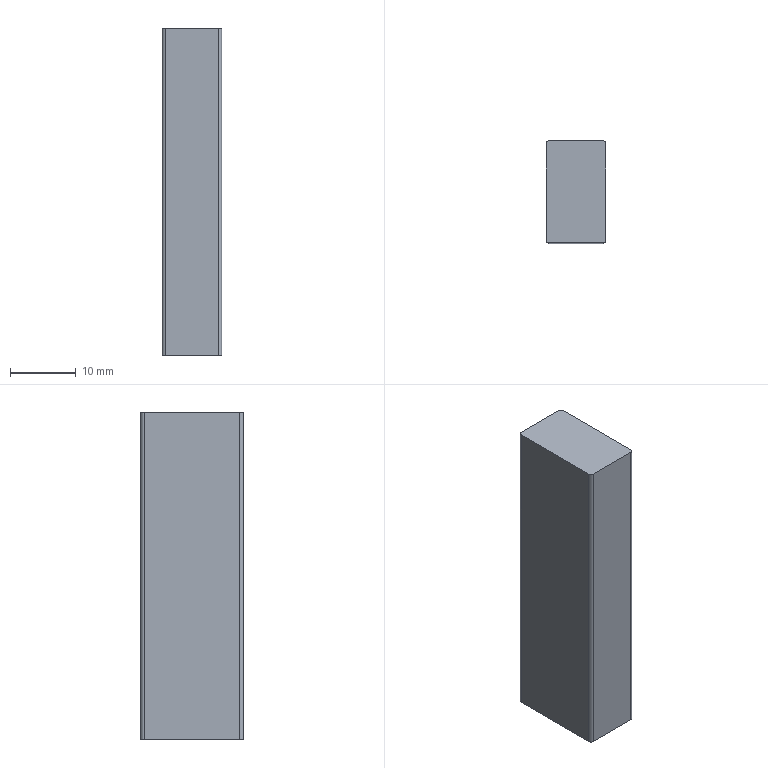Part | NX | features BREP 1 | 1 solid | 10 faces | box 9.1 x 15.637 x 50 mm | volume 7104 mm3 | plane 6 | cylinder 4 | commonest cylinder face diameters 1 x4
STEP:
#1=CARTESIAN_POINT('',(-4.05,7.819,-40.6));
#2=VERTEX_POINT('',#1);
#3=CARTESIAN_POINT('',(-4.55,7.319,-40.6));
#4=VERTEX_POINT('',#3);
#5=CARTESIAN_POINT('',(-4.05,7.319,-40.6));
#6=DIRECTION('',(0.,0.,1.));
#7=DIRECTION('',(1.,0.,0.));
#8=AXIS2_PLACEMENT_3D('',#5,#6,#7);
#9=CIRCLE('',#8,0.5);
#10=EDGE_CURVE('',#2,#4,#9,.T.);
#11=ORIENTED_EDGE('',*,*,#10,.F.);
#12=CARTESIAN_POINT('',(-4.05,7.819,-90.6));
#13=VERTEX_POINT('',#12);
#14=CARTESIAN_POINT('',(-4.05,7.819,-90.6));
#15=DIRECTION('',(0.,0.,1.));
#16=VECTOR('',#15,1000.);
#17=LINE('',#14,#16);
#18=EDGE_CURVE('',#13,#2,#17,.T.);
#19=ORIENTED_EDGE('',*,*,#18,.F.);
#20=CARTESIAN_POINT('',(-4.55,7.319,-90.6));
#21=VERTEX_POINT('',#20);
#22=CARTESIAN_POINT('',(-4.05,7.319,-90.6));
#23=DIRECTION('',(0.,0.,1.));
#24=DIRECTION('',(1.,0.,0.));
#25=AXIS2_PLACEMENT_3D('',#22,#23,#24);
#26=CIRCLE('',#25,0.5);
#27=EDGE_CURVE('',#13,#21,#26,.T.);
#28=ORIENTED_EDGE('',*,*,#27,.T.);
#29=CARTESIAN_POINT('',(-4.55,7.319,-90.6));
#30=DIRECTION('',(0.,0.,1.));
#31=VECTOR('',#30,1000.);
#32=LINE('',#29,#31);
#33=EDGE_CURVE('',#21,#4,#32,.T.);
#34=ORIENTED_EDGE('',*,*,#33,.T.);
#35=EDGE_LOOP('',(#11,#19,#28,#34));
#36=FACE_BOUND('',#35,.T.);
#37=CARTESIAN_POINT('',(-4.05,7.319,-90.6));
#38=DIRECTION('',(0.,0.,1.));
#39=DIRECTION('',(-1.,0.,0.));
#40=AXIS2_PLACEMENT_3D('',#37,#38,#39);
#41=CYLINDRICAL_SURFACE('',#40,0.5);
#42=ADVANCED_FACE('',(#36),#41,.T.);
#43=CARTESIAN_POINT('',(-4.55,-7.319,-40.6));
#44=VERTEX_POINT('',#43);
#45=CARTESIAN_POINT('',(-4.55,-7.319,-40.6));
#46=DIRECTION('',(0.,1.,0.));
#47=VECTOR('',#46,1000.);
#48=LINE('',#45,#47);
#49=EDGE_CURVE('',#44,#4,#48,.T.);
#50=ORIENTED_EDGE('',*,*,#49,.T.);
#51=ORIENTED_EDGE('',*,*,#33,.F.);
#52=CARTESIAN_POINT('',(-4.55,-7.319,-90.6));
#53=VERTEX_POINT('',#52);
#54=CARTESIAN_POINT('',(-4.55,-7.319,-90.6));
#55=DIRECTION('',(0.,1.,0.));
#56=VECTOR('',#55,1000.);
#57=LINE('',#54,#56);
#58=EDGE_CURVE('',#53,#21,#57,.T.);
#59=ORIENTED_EDGE('',*,*,#58,.F.);
#60=CARTESIAN_POINT('',(-4.55,-7.319,-90.6));
#61=DIRECTION('',(0.,0.,1.));
#62=VECTOR('',#61,1000.);
#63=LINE('',#60,#62);
#64=EDGE_CURVE('',#53,#44,#63,.T.);
#65=ORIENTED_EDGE('',*,*,#64,.T.);
#66=EDGE_LOOP('',(#50,#51,#59,#65));
#67=FACE_BOUND('',#66,.T.);
#68=CARTESIAN_POINT('',(-4.55,-7.319,-90.6));
#69=DIRECTION('',(1.,0.,0.));
#70=DIRECTION('',(0.,-1.,0.));
#71=AXIS2_PLACEMENT_3D('',#68,#69,#70);
#72=PLANE('',#71);
#73=ADVANCED_FACE('',(#67),#72,.F.);
#74=CARTESIAN_POINT('',(-4.05,-7.819,-40.6));
#75=VERTEX_POINT('',#74);
#76=CARTESIAN_POINT('',(-4.05,-7.319,-40.6));
#77=DIRECTION('',(0.,0.,1.));
#78=DIRECTION('',(1.,0.,0.));
#79=AXIS2_PLACEMENT_3D('',#76,#77,#78);
#80=CIRCLE('',#79,0.5);
#81=EDGE_CURVE('',#44,#75,#80,.T.);
#82=ORIENTED_EDGE('',*,*,#81,.F.);
#83=ORIENTED_EDGE('',*,*,#64,.F.);
#84=CARTESIAN_POINT('',(-4.05,-7.819,-90.6));
#85=VERTEX_POINT('',#84);
#86=CARTESIAN_POINT('',(-4.05,-7.319,-90.6));
#87=DIRECTION('',(0.,0.,1.));
#88=DIRECTION('',(1.,0.,0.));
#89=AXIS2_PLACEMENT_3D('',#86,#87,#88);
#90=CIRCLE('',#89,0.5);
#91=EDGE_CURVE('',#53,#85,#90,.T.);
#92=ORIENTED_EDGE('',*,*,#91,.T.);
#93=CARTESIAN_POINT('',(-4.05,-7.819,-90.6));
#94=DIRECTION('',(0.,0.,1.));
#95=VECTOR('',#94,1000.);
#96=LINE('',#93,#95);
#97=EDGE_CURVE('',#85,#75,#96,.T.);
#98=ORIENTED_EDGE('',*,*,#97,.T.);
#99=EDGE_LOOP('',(#82,#83,#92,#98));
#100=FACE_BOUND('',#99,.T.);
#101=CARTESIAN_POINT('',(-4.05,-7.319,-90.6));
#102=DIRECTION('',(0.,0.,1.));
#103=DIRECTION('',(-1.,0.,0.));
#104=AXIS2_PLACEMENT_3D('',#101,#102,#103);
#105=CYLINDRICAL_SURFACE('',#104,0.5);
#106=ADVANCED_FACE('',(#100),#105,.T.);
#107=CARTESIAN_POINT('',(4.05,-7.819,-40.6));
#108=VERTEX_POINT('',#107);
#109=CARTESIAN_POINT('',(4.05,-7.819,-40.6));
#110=DIRECTION('',(-1.,0.,0.));
#111=VECTOR('',#110,1000.);
#112=LINE('',#109,#111);
#113=EDGE_CURVE('',#108,#75,#112,.T.);
#114=ORIENTED_EDGE('',*,*,#113,.T.);
#115=ORIENTED_EDGE('',*,*,#97,.F.);
#116=CARTESIAN_POINT('',(4.05,-7.819,-90.6));
#117=VERTEX_POINT('',#116);
#118=CARTESIAN_POINT('',(4.05,-7.819,-90.6));
#119=DIRECTION('',(-1.,0.,0.));
#120=VECTOR('',#119,1000.);
#121=LINE('',#118,#120);
#122=EDGE_CURVE('',#117,#85,#121,.T.);
#123=ORIENTED_EDGE('',*,*,#122,.F.);
#124=CARTESIAN_POINT('',(4.05,-7.819,-90.6));
#125=DIRECTION('',(0.,0.,1.));
#126=VECTOR('',#125,1000.);
#127=LINE('',#124,#126);
#128=EDGE_CURVE('',#117,#108,#127,.T.);
#129=ORIENTED_EDGE('',*,*,#128,.T.);
#130=EDGE_LOOP('',(#114,#115,#123,#129));
#131=FACE_BOUND('',#130,.T.);
#132=CARTESIAN_POINT('',(4.05,-7.819,-90.6));
#133=DIRECTION('',(0.,1.,0.));
#134=DIRECTION('',(0.,0.,-1.));
#135=AXIS2_PLACEMENT_3D('',#132,#133,#134);
#136=PLANE('',#135);
#137=ADVANCED_FACE('',(#131),#136,.F.);
#138=CARTESIAN_POINT('',(4.55,-7.319,-40.6));
#139=VERTEX_POINT('',#138);
#140=CARTESIAN_POINT('',(4.05,-7.319,-40.6));
#141=DIRECTION('',(0.,0.,1.));
#142=DIRECTION('',(1.,0.,0.));
#143=AXIS2_PLACEMENT_3D('',#140,#141,#142);
#144=CIRCLE('',#143,0.5);
#145=EDGE_CURVE('',#108,#139,#144,.T.);
#146=ORIENTED_EDGE('',*,*,#145,.F.);
#147=ORIENTED_EDGE('',*,*,#128,.F.);
#148=CARTESIAN_POINT('',(4.55,-7.319,-90.6));
#149=VERTEX_POINT('',#148);
#150=CARTESIAN_POINT('',(4.05,-7.319,-90.6));
#151=DIRECTION('',(0.,0.,1.));
#152=DIRECTION('',(1.,0.,0.));
#153=AXIS2_PLACEMENT_3D('',#150,#151,#152);
#154=CIRCLE('',#153,0.5);
#155=EDGE_CURVE('',#117,#149,#154,.T.);
#156=ORIENTED_EDGE('',*,*,#155,.T.);
#157=CARTESIAN_POINT('',(4.55,-7.319,-90.6));
#158=DIRECTION('',(0.,0.,1.));
#159=VECTOR('',#158,1000.);
#160=LINE('',#157,#159);
#161=EDGE_CURVE('',#149,#139,#160,.T.);
#162=ORIENTED_EDGE('',*,*,#161,.T.);
#163=EDGE_LOOP('',(#146,#147,#156,#162));
#164=FACE_BOUND('',#163,.T.);
#165=CARTESIAN_POINT('',(4.05,-7.319,-90.6));
#166=DIRECTION('',(0.,0.,1.));
#167=DIRECTION('',(-1.,0.,0.));
#168=AXIS2_PLACEMENT_3D('',#165,#166,#167);
#169=CYLINDRICAL_SURFACE('',#168,0.5);
#170=ADVANCED_FACE('',(#164),#169,.T.);
#171=CARTESIAN_POINT('',(4.55,7.319,-40.6));
#172=VERTEX_POINT('',#171);
#173=CARTESIAN_POINT('',(4.55,7.319,-40.6));
#174=DIRECTION('',(0.,-1.,0.));
#175=VECTOR('',#174,1000.);
#176=LINE('',#173,#175);
#177=EDGE_CURVE('',#172,#139,#176,.T.);
#178=ORIENTED_EDGE('',*,*,#177,.T.);
#179=ORIENTED_EDGE('',*,*,#161,.F.);
#180=CARTESIAN_POINT('',(4.55,7.319,-90.6));
#181=VERTEX_POINT('',#180);
#182=CARTESIAN_POINT('',(4.55,7.319,-90.6));
#183=DIRECTION('',(0.,-1.,0.));
#184=VECTOR('',#183,1000.);
#185=LINE('',#182,#184);
#186=EDGE_CURVE('',#181,#149,#185,.T.);
#187=ORIENTED_EDGE('',*,*,#186,.F.);
#188=CARTESIAN_POINT('',(4.55,7.319,-90.6));
#189=DIRECTION('',(0.,0.,1.));
#190=VECTOR('',#189,1000.);
#191=LINE('',#188,#190);
#192=EDGE_CURVE('',#181,#172,#191,.T.);
#193=ORIENTED_EDGE('',*,*,#192,.T.);
#194=EDGE_LOOP('',(#178,#179,#187,#193));
#195=FACE_BOUND('',#194,.T.);
#196=CARTESIAN_POINT('',(4.55,7.319,-90.6));
#197=DIRECTION('',(-1.,0.,0.));
#198=DIRECTION('',(0.,0.,-1.));
#199=AXIS2_PLACEMENT_3D('',#196,#197,#198);
#200=PLANE('',#199);
#201=ADVANCED_FACE('',(#195),#200,.F.);
#202=CARTESIAN_POINT('',(4.05,7.819,-40.6));
#203=VERTEX_POINT('',#202);
#204=CARTESIAN_POINT('',(4.05,7.319,-40.6));
#205=DIRECTION('',(0.,0.,1.));
#206=DIRECTION('',(1.,0.,0.));
#207=AXIS2_PLACEMENT_3D('',#204,#205,#206);
#208=CIRCLE('',#207,0.5);
#209=EDGE_CURVE('',#172,#203,#208,.T.);
#210=ORIENTED_EDGE('',*,*,#209,.F.);
#211=ORIENTED_EDGE('',*,*,#192,.F.);
#212=CARTESIAN_POINT('',(4.05,7.819,-90.6));
#213=VERTEX_POINT('',#212);
#214=CARTESIAN_POINT('',(4.05,7.319,-90.6));
#215=DIRECTION('',(0.,0.,1.));
#216=DIRECTION('',(1.,0.,0.));
#217=AXIS2_PLACEMENT_3D('',#214,#215,#216);
#218=CIRCLE('',#217,0.5);
#219=EDGE_CURVE('',#181,#213,#218,.T.);
#220=ORIENTED_EDGE('',*,*,#219,.T.);
#221=CARTESIAN_POINT('',(4.05,7.819,-90.6));
#222=DIRECTION('',(0.,0.,1.));
#223=VECTOR('',#222,1000.);
#224=LINE('',#221,#223);
#225=EDGE_CURVE('',#213,#203,#224,.T.);
#226=ORIENTED_EDGE('',*,*,#225,.T.);
#227=EDGE_LOOP('',(#210,#211,#220,#226));
#228=FACE_BOUND('',#227,.T.);
#229=CARTESIAN_POINT('',(4.05,7.319,-90.6));
#230=DIRECTION('',(0.,0.,1.));
#231=DIRECTION('',(-1.,0.,0.));
#232=AXIS2_PLACEMENT_3D('',#229,#230,#231);
#233=CYLINDRICAL_SURFACE('',#232,0.5);
#234=ADVANCED_FACE('',(#228),#233,.T.);
#235=CARTESIAN_POINT('',(-4.05,7.819,-40.6));
#236=DIRECTION('',(1.,0.,0.));
#237=VECTOR('',#236,1000.);
#238=LINE('',#235,#237);
#239=EDGE_CURVE('',#2,#203,#238,.T.);
#240=ORIENTED_EDGE('',*,*,#239,.T.);
#241=ORIENTED_EDGE('',*,*,#225,.F.);
#242=CARTESIAN_POINT('',(-4.05,7.819,-90.6));
#243=DIRECTION('',(1.,0.,0.));
#244=VECTOR('',#243,1000.);
#245=LINE('',#242,#244);
#246=EDGE_CURVE('',#13,#213,#245,.T.);
#247=ORIENTED_EDGE('',*,*,#246,.F.);
#248=ORIENTED_EDGE('',*,*,#18,.T.);
#249=EDGE_LOOP('',(#240,#241,#247,#248));
#250=FACE_BOUND('',#249,.T.);
#251=CARTESIAN_POINT('',(-4.05,7.819,-90.6));
#252=DIRECTION('',(0.,-1.,0.));
#253=DIRECTION('',(0.,0.,1.));
#254=AXIS2_PLACEMENT_3D('',#251,#252,#253);
#255=PLANE('',#254);
#256=ADVANCED_FACE('',(#250),#255,.F.);
#257=ORIENTED_EDGE('',*,*,#27,.F.);
#258=ORIENTED_EDGE('',*,*,#246,.T.);
#259=ORIENTED_EDGE('',*,*,#219,.F.);
#260=ORIENTED_EDGE('',*,*,#186,.T.);
#261=ORIENTED_EDGE('',*,*,#155,.F.);
#262=ORIENTED_EDGE('',*,*,#122,.T.);
#263=ORIENTED_EDGE('',*,*,#91,.F.);
#264=ORIENTED_EDGE('',*,*,#58,.T.);
#265=EDGE_LOOP('',(#257,#258,#259,#260,#261,#262,#263,#264));
#266=FACE_BOUND('',#265,.T.);
#267=CARTESIAN_POINT('',(-4.05,7.319,-90.6));
#268=DIRECTION('',(0.,0.,1.));
#269=DIRECTION('',(-1.,0.,0.));
#270=AXIS2_PLACEMENT_3D('',#267,#268,#269);
#271=PLANE('',#270);
#272=ADVANCED_FACE('',(#266),#271,.F.);
#273=ORIENTED_EDGE('',*,*,#10,.T.);
#274=ORIENTED_EDGE('',*,*,#49,.F.);
#275=ORIENTED_EDGE('',*,*,#81,.T.);
#276=ORIENTED_EDGE('',*,*,#113,.F.);
#277=ORIENTED_EDGE('',*,*,#145,.T.);
#278=ORIENTED_EDGE('',*,*,#177,.F.);
#279=ORIENTED_EDGE('',*,*,#209,.T.);
#280=ORIENTED_EDGE('',*,*,#239,.F.);
#281=EDGE_LOOP('',(#273,#274,#275,#276,#277,#278,#279,#280));
#282=FACE_BOUND('',#281,.T.);
#283=CARTESIAN_POINT('',(-4.05,7.319,-40.6));
#284=DIRECTION('',(0.,0.,1.));
#285=DIRECTION('',(-1.,0.,0.));
#286=AXIS2_PLACEMENT_3D('',#283,#284,#285);
#287=PLANE('',#286);
#288=ADVANCED_FACE('',(#282),#287,.T.);
#289=CLOSED_SHELL('',(#42,#73,#106,#137,#170,#201,#234,#256,#272,#288));
#290=MANIFOLD_SOLID_BREP('',#289);
#291=(LENGTH_UNIT()NAMED_UNIT(*)SI_UNIT(.MILLI.,.METRE.));
#292=UNCERTAINTY_MEASURE_WITH_UNIT(LENGTH_MEASURE(0.00001),#291,'','');
#293=(NAMED_UNIT(*)PLANE_ANGLE_UNIT()SI_UNIT($,.RADIAN.));
#294=(NAMED_UNIT(*)SI_UNIT($,.STERADIAN.)SOLID_ANGLE_UNIT());
#295=(GEOMETRIC_REPRESENTATION_CONTEXT(3)GLOBAL_UNCERTAINTY_ASSIGNED_CONTEXT((#292))GLOBAL_UNIT_ASSIGNED_CONTEXT((#291,#293,#294))REPRESENTATION_CONTEXT('',''));
#296=ADVANCED_BREP_SHAPE_REPRESENTATION('',(#290),#295);